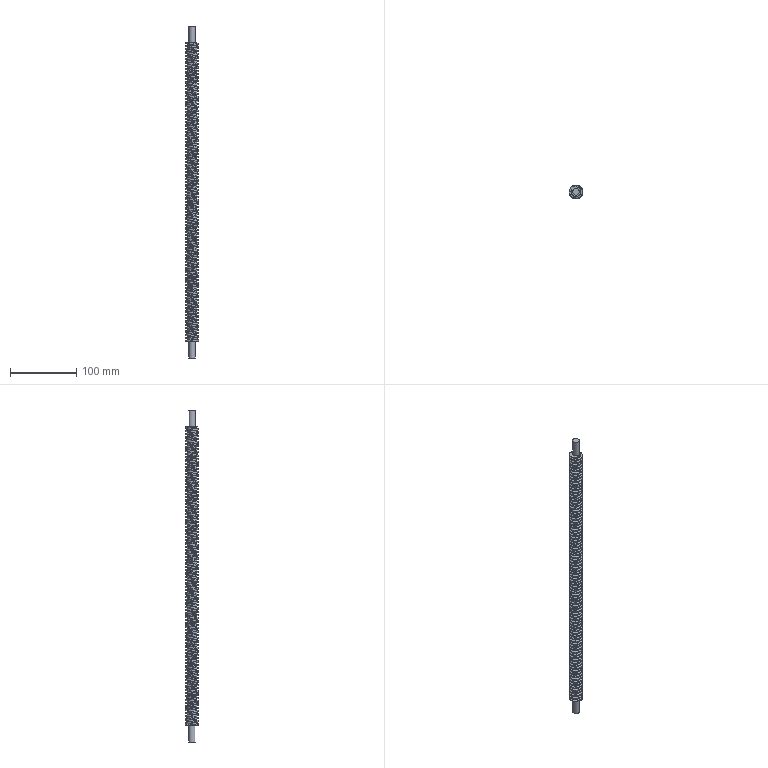Part | NX | features DATUM_CSYS 6, EXTRUDE 5, SKETCH 5, DATUM_PLANE 3, THREADS 1 | 1 solid | 11 faces | box 20 x 20 x 500 mm | volume 99158 mm3 | plane 5 | cylinder 4 | spline 2 | commonest cylinder face diameters 10 x2 14.5 x1 20 x1